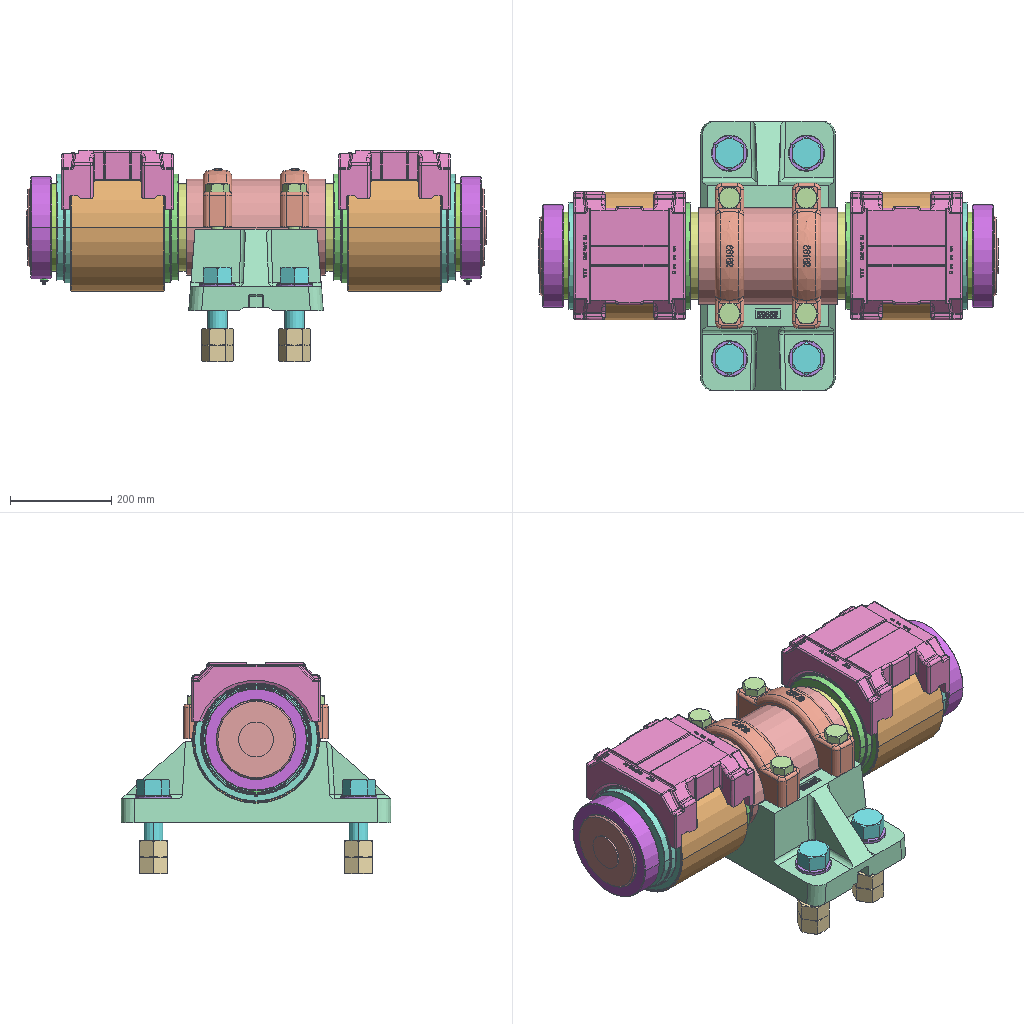Assembly | SolidWorks | 12 different items | 33 placed | box 910 x 533 x 418 mm
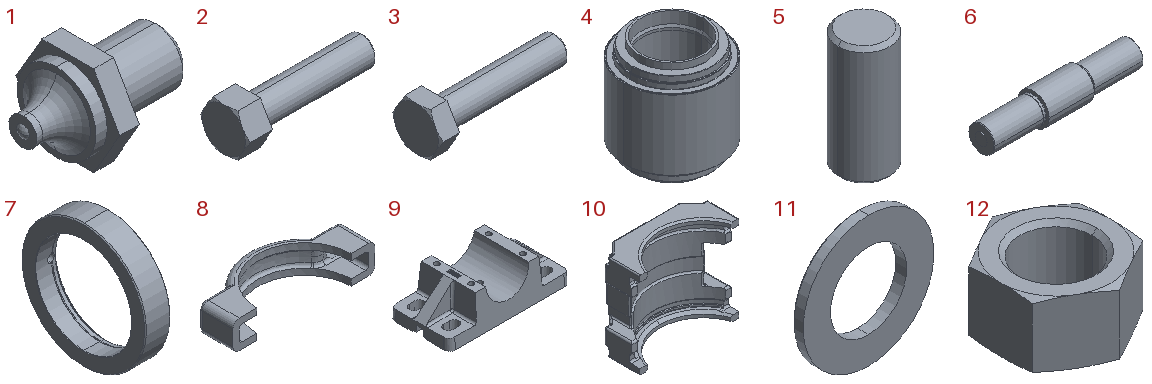Parts list (item | quantity | size | volume | features):
1 | x2 | - | - | features RefSurface 2
2 | x4 | 185.42 x 65.991 x 57.15 mm | 265435 mm3 | features RevCut 4, Chamfer 1, Extrusion 1, Fillet 1, LPattern 1, Revolution 1
3 | x4 | 131.3 x 47.343 x 41 mm | 82460 mm3 | features RevCut 4, Chamfer 1, Extrusion 1, Fillet 1, LPattern 1, Revolution 1
4 | x2 | 252.413 x 252.413 x 273.304 mm | 4431426 mm3 | features Revolution 12, CirPattern 2, Fillet 2, Chamfer 1, Cut 1
5 | x1 | 22.225 x 22.225 x 50.8 mm | 19553 mm3 | features Chamfer 1, Extrusion 1
6 | x1 | 909.904 x 190.424 x 190.424 mm | 20016200 mm3 | features Chamfer 2, Cut 1, Fillet 1, Revolution 1
7 | x2 | 41.402 x 203.2 x 203.2 mm | 502742 mm3 | features Chamfer 2, 3DProfileFeature 1, HoleWzd 1, Revolution 1
8 | x2 | 287 x 115.887 x 57.15 mm | 415427 mm3 | features Fillet 6, Boss 1, Cut 1, Extrusion 1, Revolution 1, Shell 1
9 | x1 | 533.4 x 265.974 x 161.862 mm | 11273677 mm3 | features Cut 6, MirrorPattern 4, Boss 3, Fillet 3, 3DProfileFeature 1, Extrusion 1, HoleWzd 1, RevCut 1
10 | x2 | 253.206 x 115.888 x 220.663 mm | 2117949 mm3 | features Fillet 8, Cut 5, Draft 4, MirrorPattern 3, Boss 2, RevCut 2, Extrusion 1
11 | x4 | 72 x 6 x 72 mm | 16004 mm3 | features Revolution 1
12 | x8 | 56.219 x 64.769 x 32.544 mm | 53250 mm3 | features Cut 2, Chamfer 1, Extrusion 1
Mates (type | each side: item.copy, entity, surface, feature):
Concentric | 6.1 face cylinder Revolve1 | 4.1 face cylinder Revolve8
Concentric | 6.1 face cylinder Revolve1 | 7.1 face cylinder Revolve1
Concentric | 6.1 face cylinder Revolve1 | 7.2 face cylinder Revolve1
Coincident | 7.1 select_type:24 | 7.2 select_type:24
Concentric | 6.1 face cylinder Revolve1 | 9.1 face cylinder Cut-Extrude6
Coincident | 9.1 plane | assembly plane
Concentric | 6.1 face cylinder Revolve1 | 8.1 face cylinder Extrude1
Parallel | 9.1 face plane Extrude2 | 8.1 face plane Extrude1
Concentric | 6.1 face cylinder Revolve1 | 8.2 face cylinder Extrude1
Parallel | 9.1 face plane Extrude2 | 8.2 face plane Extrude1
Concentric | 6.1 face cylinder Cut-Extrude1 | 5.1 face cylinder Extrude1
Coincident | 6.1 face plane Cut-Extrude1 | 5.1 face plane Extrude1
Concentric | 9.1 face cylinder Cut-Revolve1 | 5.1 face cylinder Extrude1
DistanceDim | 8.1 plane | assembly plane
DistanceDim | 8.2 plane | assembly plane
Concentric | 8.1 face cylinder Cut-Extrude1 | 3.1 face cylinder Boss-Revolve1
Coincident | 8.1 face plane Extrude1 | 3.1 face plane Base-Extrude
Parallel | 8.1 face plane Extrude1 | 3.1 face plane Base-Extrude
Coincident | 7.2 plane | assembly plane
Coincident | 6.1 face plane Revolve1 | 4.1 face plane Revolve10
Concentric | 4.1 face cylinder Revolve8 | 10.1 face cylinder Cut-Revolve1
Coincident | 4.1 plane | 10.1 plane
Concentric | 6.1 face cylinder Revolve1 | 4.2 face cylinder Revolve8
Coincident | 6.1 face plane Revolve1 | 4.2 face plane Revolve10
Concentric | 4.2 face cylinder Revolve8 | 10.2 face cylinder Cut-Revolve1
Coincident | 4.2 plane | 10.2 plane
Parallel | 9.1 face plane Extrude2 | 10.1 face plane Cut-Extrude2
Coincident | 4.2 face plane Revolve3 | 7.1 face plane Revolve1
Coincident | 4.1 face plane Revolve3 | 7.2 face plane Revolve1
Coincident | 4.2 plane | 4.1 plane
Coincident | 4.2 plane | assembly plane
Concentric | 1.1 face cylinder Oil cup M10×1-1-surface1 | 7.1 face cylinder 1/8 NPT Tapped Hole1
Tangent | 7.1 face cylinder Revolve1 | 1.1 face plane Oil cup M10×1-1-surface1
Parallel | 7.1 face plane Revolve1 | 1.1 face plane Oil cup M10×1-1-surface1
Concentric | 1.2 face cylinder Oil cup M10×1-1-surface1 | 7.2 face cylinder 1/8 NPT Tapped Hole1
Tangent | 7.2 face cylinder Revolve1 | 1.2 face plane Oil cup M10×1-1-surface1
Parallel | 7.2 face plane Revolve1 | 1.2 face plane Oil cup M10×1-1-surface1
Coincident | 2.1 plane | 9.1 plane | 2 times
Concentric | 2.1 face cylinder Boss-Revolve1 | 11.1 face cylinder Base-Revolve
Coincident | 9.1 face plane Extrude1 | 11.1 face plane Base-Revolve
Coincident | 2.1 face plane Base-Extrude | 11.1 face plane Base-Revolve
Concentric | 2.1 face cylinder Boss-Revolve1 | 12.1 face cylinder Base-Extrude
DistanceDim | 9.1 face plane Cut-Extrude6 | 12.1 face plane Base-Extrude
Concentric | 2.1 face cylinder Boss-Revolve1 | 12.2 face cylinder Base-Extrude
Coincident | 12.1 face plane Base-Extrude | 12.2 face plane Base-Extrude | 2 times
Parallel | 9.1 face plane Extrude1 | 12.1 face plane Base-Extrude